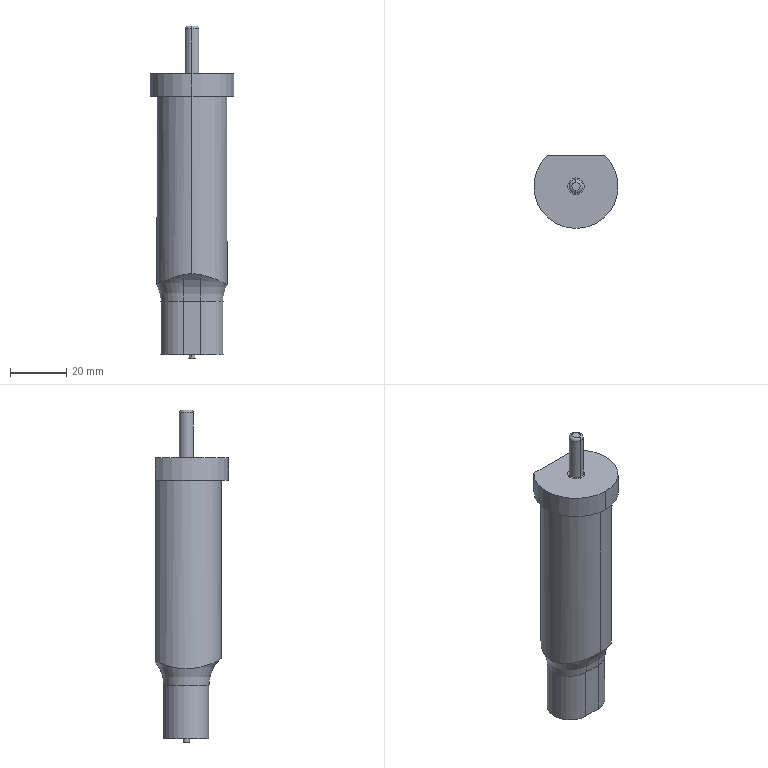Part | STEP file | 1_id3566_x_t | 1 solid | 27 faces | box 30 x 26 x 118.2 mm | volume 45235 mm3 | cylinder 14 | plane 9 | torus 4 | commonest cylinder face diameters 2.26 x2 5 x2 6 x2 16.07 x2 25 x2 26 x2
STEP:
#1=CARTESIAN_POINT('',(3206.065,143.382,20.96));
#2=VERTEX_POINT('',#1);
#3=CARTESIAN_POINT('',(3208.937,166.5,20.193));
#4=VERTEX_POINT('',#3);
#5=CARTESIAN_POINT('',(3206.065,143.382,20.96));
#6=CARTESIAN_POINT('',(3208.507,143.999,20.378));
#7=CARTESIAN_POINT('',(3210.679,145.334,19.684));
#8=CARTESIAN_POINT('',(3213.962,149.007,18.317));
#9=CARTESIAN_POINT('',(3215.071,151.383,17.64));
#10=CARTESIAN_POINT('',(3215.722,156.404,17.229));
#11=CARTESIAN_POINT('',(3215.235,159.073,17.588));
#12=CARTESIAN_POINT('',(3212.932,163.488,18.779));
#13=CARTESIAN_POINT('',(3211.138,165.312,19.533));
#14=CARTESIAN_POINT('',(3208.937,166.5,20.193));
#15=B_SPLINE_CURVE_WITH_KNOTS('',3,(#5,#6,#7,#8,#9,#10,#11,#12,#13,#14),.UNSPECIFIED.,.F.,.F.,(4,2,2,2,4),(0.,0.25,0.5,0.75,1.),.UNSPECIFIED.);
#16=EDGE_CURVE('',#2,#4,#15,.T.);
#17=ORIENTED_EDGE('',*,*,#16,.T.);
#18=CARTESIAN_POINT('',(3208.937,166.5,84.5));
#19=VERTEX_POINT('',#18);
#20=CARTESIAN_POINT('',(3208.937,166.5,38.5));
#21=DIRECTION('',(0.,0.,1.));
#22=VECTOR('',#21,1.);
#23=LINE('',#20,#22);
#24=EDGE_CURVE('',#4,#19,#23,.T.);
#25=ORIENTED_EDGE('',*,*,#24,.T.);
#26=CARTESIAN_POINT('',(3203.,143.,84.5));
#27=VERTEX_POINT('',#26);
#28=CARTESIAN_POINT('',(3203.,155.5,84.5));
#29=DIRECTION('',(0.,0.,1.));
#30=DIRECTION('',(0.,-1.,0.));
#31=AXIS2_PLACEMENT_3D('',#28,#29,#30);
#32=CIRCLE('',#31,12.5);
#33=EDGE_CURVE('',#27,#19,#32,.T.);
#34=ORIENTED_EDGE('',*,*,#33,.F.);
#35=CARTESIAN_POINT('',(3203.,143.,21.306));
#36=VERTEX_POINT('',#35);
#37=CARTESIAN_POINT('',(3203.,143.,38.5));
#38=DIRECTION('',(0.,0.,1.));
#39=VECTOR('',#38,1.);
#40=LINE('',#37,#39);
#41=EDGE_CURVE('',#36,#27,#40,.T.);
#42=ORIENTED_EDGE('',*,*,#41,.F.);
#43=CARTESIAN_POINT('',(3203.,143.,21.306));
#44=CARTESIAN_POINT('',(3204.051,143.,21.306));
#45=CARTESIAN_POINT('',(3205.073,143.131,21.197));
#46=CARTESIAN_POINT('',(3206.065,143.382,20.96));
#47=B_SPLINE_CURVE_WITH_KNOTS('',3,(#43,#44,#45,#46),.UNSPECIFIED.,.F.,.F.,(4,4),(0.,1.),.UNSPECIFIED.);
#48=EDGE_CURVE('',#36,#2,#47,.T.);
#49=ORIENTED_EDGE('',*,*,#48,.T.);
#50=EDGE_LOOP('',(#17,#25,#34,#42,#49));
#51=FACE_OUTER_BOUND('',#50,.T.);
#52=CARTESIAN_POINT('',(3203.,155.5,38.5));
#53=DIRECTION('',(0.,0.,-1.));
#54=DIRECTION('',(0.,1.,0.));
#55=AXIS2_PLACEMENT_3D('',#52,#53,#54);
#56=CYLINDRICAL_SURFACE('',#55,12.5);
#57=ADVANCED_FACE('',(#51),#56,.T.);
#58=CARTESIAN_POINT('',(3203.,140.5,84.5));
#59=VERTEX_POINT('',#58);
#60=CARTESIAN_POINT('',(3213.198,166.5,84.5));
#61=VERTEX_POINT('',#60);
#62=CARTESIAN_POINT('',(3203.,155.5,84.5));
#63=DIRECTION('',(0.,0.,1.));
#64=DIRECTION('',(0.,-1.,0.));
#65=AXIS2_PLACEMENT_3D('',#62,#63,#64);
#66=CIRCLE('',#65,15.);
#67=EDGE_CURVE('',#59,#61,#66,.T.);
#68=ORIENTED_EDGE('',*,*,#67,.T.);
#69=CARTESIAN_POINT('',(3213.198,166.5,92.5));
#70=VERTEX_POINT('',#69);
#71=CARTESIAN_POINT('',(3213.198,166.5,88.5));
#72=DIRECTION('',(0.,0.,1.));
#73=VECTOR('',#72,1.);
#74=LINE('',#71,#73);
#75=EDGE_CURVE('',#61,#70,#74,.T.);
#76=ORIENTED_EDGE('',*,*,#75,.T.);
#77=CARTESIAN_POINT('',(3203.,140.5,92.5));
#78=VERTEX_POINT('',#77);
#79=CARTESIAN_POINT('',(3203.,155.5,92.5));
#80=DIRECTION('',(0.,0.,1.));
#81=DIRECTION('',(0.,-1.,0.));
#82=AXIS2_PLACEMENT_3D('',#79,#80,#81);
#83=CIRCLE('',#82,15.);
#84=EDGE_CURVE('',#78,#70,#83,.T.);
#85=ORIENTED_EDGE('',*,*,#84,.F.);
#86=CARTESIAN_POINT('',(3203.,140.5,88.5));
#87=DIRECTION('',(0.,0.,1.));
#88=VECTOR('',#87,1.);
#89=LINE('',#86,#88);
#90=EDGE_CURVE('',#59,#78,#89,.T.);
#91=ORIENTED_EDGE('',*,*,#90,.F.);
#92=EDGE_LOOP('',(#68,#76,#85,#91));
#93=FACE_OUTER_BOUND('',#92,.T.);
#94=CARTESIAN_POINT('',(3203.,155.5,88.5));
#95=DIRECTION('',(0.,0.,-1.));
#96=DIRECTION('',(0.,1.,0.));
#97=AXIS2_PLACEMENT_3D('',#94,#95,#96);
#98=CYLINDRICAL_SURFACE('',#97,15.);
#99=ADVANCED_FACE('',(#93),#98,.T.);
#100=CARTESIAN_POINT('',(3192.802,166.5,92.5));
#101=VERTEX_POINT('',#100);
#102=CARTESIAN_POINT('',(3203.,155.5,92.5));
#103=DIRECTION('',(0.,0.,1.));
#104=DIRECTION('',(0.,-1.,0.));
#105=AXIS2_PLACEMENT_3D('',#102,#103,#104);
#106=CIRCLE('',#105,15.);
#107=EDGE_CURVE('',#101,#78,#106,.T.);
#108=ORIENTED_EDGE('',*,*,#107,.F.);
#109=CARTESIAN_POINT('',(3192.802,166.5,84.5));
#110=VERTEX_POINT('',#109);
#111=CARTESIAN_POINT('',(3192.802,166.5,88.5));
#112=DIRECTION('',(0.,0.,1.));
#113=VECTOR('',#112,1.);
#114=LINE('',#111,#113);
#115=EDGE_CURVE('',#110,#101,#114,.T.);
#116=ORIENTED_EDGE('',*,*,#115,.F.);
#117=CARTESIAN_POINT('',(3203.,155.5,84.5));
#118=DIRECTION('',(0.,0.,1.));
#119=DIRECTION('',(0.,-1.,0.));
#120=AXIS2_PLACEMENT_3D('',#117,#118,#119);
#121=CIRCLE('',#120,15.);
#122=EDGE_CURVE('',#110,#59,#121,.T.);
#123=ORIENTED_EDGE('',*,*,#122,.T.);
#124=ORIENTED_EDGE('',*,*,#90,.T.);
#125=EDGE_LOOP('',(#108,#116,#123,#124));
#126=FACE_OUTER_BOUND('',#125,.T.);
#127=CARTESIAN_POINT('',(3203.,155.5,88.5));
#128=DIRECTION('',(0.,0.,-1.));
#129=DIRECTION('',(0.,1.,0.));
#130=AXIS2_PLACEMENT_3D('',#127,#128,#129);
#131=CYLINDRICAL_SURFACE('',#130,15.);
#132=ADVANCED_FACE('',(#126),#131,.T.);
#133=ORIENTED_EDGE('',*,*,#122,.F.);
#134=CARTESIAN_POINT('',(3197.063,166.5,84.5));
#135=VERTEX_POINT('',#134);
#136=CARTESIAN_POINT('',(3203.,166.5,84.5));
#137=DIRECTION('',(-1.,0.,0.));
#138=VECTOR('',#137,1.);
#139=LINE('',#136,#138);
#140=EDGE_CURVE('',#135,#110,#139,.T.);
#141=ORIENTED_EDGE('',*,*,#140,.F.);
#142=CARTESIAN_POINT('',(3203.,155.5,84.5));
#143=DIRECTION('',(0.,0.,1.));
#144=DIRECTION('',(0.,-1.,0.));
#145=AXIS2_PLACEMENT_3D('',#142,#143,#144);
#146=CIRCLE('',#145,12.5);
#147=EDGE_CURVE('',#135,#27,#146,.T.);
#148=ORIENTED_EDGE('',*,*,#147,.T.);
#149=ORIENTED_EDGE('',*,*,#33,.T.);
#150=CARTESIAN_POINT('',(3203.,166.5,84.5));
#151=DIRECTION('',(-1.,0.,0.));
#152=VECTOR('',#151,1.);
#153=LINE('',#150,#152);
#154=EDGE_CURVE('',#61,#19,#153,.T.);
#155=ORIENTED_EDGE('',*,*,#154,.F.);
#156=ORIENTED_EDGE('',*,*,#67,.F.);
#157=EDGE_LOOP('',(#133,#141,#148,#149,#155,#156));
#158=FACE_OUTER_BOUND('',#157,.T.);
#159=CARTESIAN_POINT('',(3203.,141.75,84.5));
#160=DIRECTION('',(0.,0.,-1.));
#161=DIRECTION('',(0.,-1.,0.));
#162=AXIS2_PLACEMENT_3D('',#159,#160,#161);
#163=PLANE('',#162);
#164=ADVANCED_FACE('',(#158),#163,.T.);
#165=CARTESIAN_POINT('',(3206.065,166.5,19.764));
#166=VERTEX_POINT('',#165);
#167=CARTESIAN_POINT('',(3206.065,166.5,19.764));
#168=CARTESIAN_POINT('',(3207.044,166.5,19.764));
#169=CARTESIAN_POINT('',(3207.998,166.5,19.929));
#170=CARTESIAN_POINT('',(3208.937,166.5,20.193));
#171=B_SPLINE_CURVE_WITH_KNOTS('',3,(#167,#168,#169,#170),.UNSPECIFIED.,.F.,.F.,(4,4),(0.,1.),.UNSPECIFIED.);
#172=EDGE_CURVE('',#166,#4,#171,.T.);
#173=ORIENTED_EDGE('',*,*,#172,.T.);
#174=ORIENTED_EDGE('',*,*,#16,.F.);
#175=CARTESIAN_POINT('',(3206.065,147.465,11.5));
#176=VERTEX_POINT('',#175);
#177=CARTESIAN_POINT('',(3206.065,134.465,11.5));
#178=DIRECTION('',(-1.,0.,0.));
#179=DIRECTION('',(0.,-1.,0.));
#180=AXIS2_PLACEMENT_3D('',#177,#178,#179);
#181=CIRCLE('',#180,13.);
#182=EDGE_CURVE('',#2,#176,#181,.T.);
#183=ORIENTED_EDGE('',*,*,#182,.T.);
#184=CARTESIAN_POINT('',(3206.065,163.535,11.5));
#185=VERTEX_POINT('',#184);
#186=CARTESIAN_POINT('',(3206.065,155.5,11.5));
#187=DIRECTION('',(0.,0.,-1.));
#188=DIRECTION('',(0.,1.,0.));
#189=AXIS2_PLACEMENT_3D('',#186,#187,#188);
#190=CIRCLE('',#189,8.035);
#191=EDGE_CURVE('',#185,#176,#190,.T.);
#192=ORIENTED_EDGE('',*,*,#191,.F.);
#193=CARTESIAN_POINT('',(3206.065,176.535,11.5));
#194=DIRECTION('',(1.,0.,0.));
#195=DIRECTION('',(0.,1.,0.));
#196=AXIS2_PLACEMENT_3D('',#193,#194,#195);
#197=CIRCLE('',#196,13.);
#198=EDGE_CURVE('',#166,#185,#197,.T.);
#199=ORIENTED_EDGE('',*,*,#198,.F.);
#200=EDGE_LOOP('',(#173,#174,#183,#192,#199));
#201=FACE_OUTER_BOUND('',#200,.T.);
#202=CARTESIAN_POINT('',(3206.065,155.5,11.5));
#203=DIRECTION('',(0.,0.,-1.));
#204=DIRECTION('',(0.,1.,0.));
#205=AXIS2_PLACEMENT_3D('',#202,#203,#204);
#206=TOROIDAL_SURFACE('',#205,21.035,13.);
#207=ADVANCED_FACE('',(#201),#206,.F.);
#208=CARTESIAN_POINT('',(3199.935,166.5,19.764));
#209=VERTEX_POINT('',#208);
#210=CARTESIAN_POINT('',(3178.,166.5,19.764));
#211=DIRECTION('',(-1.,0.,0.));
#212=VECTOR('',#211,1.);
#213=LINE('',#210,#212);
#214=EDGE_CURVE('',#166,#209,#213,.T.);
#215=ORIENTED_EDGE('',*,*,#214,.F.);
#216=ORIENTED_EDGE('',*,*,#198,.T.);
#217=CARTESIAN_POINT('',(3199.935,163.535,11.5));
#218=VERTEX_POINT('',#217);
#219=CARTESIAN_POINT('',(3178.,163.535,11.5));
#220=DIRECTION('',(1.,0.,0.));
#221=VECTOR('',#220,1.);
#222=LINE('',#219,#221);
#223=EDGE_CURVE('',#218,#185,#222,.T.);
#224=ORIENTED_EDGE('',*,*,#223,.F.);
#225=CARTESIAN_POINT('',(3199.935,176.535,11.5));
#226=DIRECTION('',(-1.,0.,0.));
#227=DIRECTION('',(0.,1.,0.));
#228=AXIS2_PLACEMENT_3D('',#225,#226,#227);
#229=CIRCLE('',#228,13.);
#230=EDGE_CURVE('',#218,#209,#229,.T.);
#231=ORIENTED_EDGE('',*,*,#230,.T.);
#232=EDGE_LOOP('',(#215,#216,#224,#231));
#233=FACE_OUTER_BOUND('',#232,.T.);
#234=CARTESIAN_POINT('',(3178.,176.535,11.5));
#235=DIRECTION('',(-1.,0.,0.));
#236=DIRECTION('',(0.,1.,0.));
#237=AXIS2_PLACEMENT_3D('',#234,#235,#236);
#238=CYLINDRICAL_SURFACE('',#237,13.);
#239=ADVANCED_FACE('',(#233),#238,.F.);
#240=CARTESIAN_POINT('',(3197.063,166.5,20.193));
#241=VERTEX_POINT('',#240);
#242=CARTESIAN_POINT('',(3197.063,166.5,20.193));
#243=CARTESIAN_POINT('',(3198.002,166.5,19.929));
#244=CARTESIAN_POINT('',(3198.956,166.5,19.764));
#245=CARTESIAN_POINT('',(3199.935,166.5,19.764));
#246=B_SPLINE_CURVE_WITH_KNOTS('',3,(#242,#243,#244,#245),.UNSPECIFIED.,.F.,.F.,(4,4),(0.,1.),.UNSPECIFIED.);
#247=EDGE_CURVE('',#241,#209,#246,.T.);
#248=ORIENTED_EDGE('',*,*,#247,.T.);
#249=ORIENTED_EDGE('',*,*,#230,.F.);
#250=CARTESIAN_POINT('',(3199.935,147.465,11.5));
#251=VERTEX_POINT('',#250);
#252=CARTESIAN_POINT('',(3199.935,155.5,11.5));
#253=DIRECTION('',(0.,0.,1.));
#254=DIRECTION('',(0.,1.,0.));
#255=AXIS2_PLACEMENT_3D('',#252,#253,#254);
#256=CIRCLE('',#255,8.035);
#257=EDGE_CURVE('',#218,#251,#256,.T.);
#258=ORIENTED_EDGE('',*,*,#257,.T.);
#259=CARTESIAN_POINT('',(3199.935,143.382,20.96));
#260=VERTEX_POINT('',#259);
#261=CARTESIAN_POINT('',(3199.935,134.465,11.5));
#262=DIRECTION('',(1.,0.,0.));
#263=DIRECTION('',(0.,-1.,0.));
#264=AXIS2_PLACEMENT_3D('',#261,#262,#263);
#265=CIRCLE('',#264,13.);
#266=EDGE_CURVE('',#251,#260,#265,.T.);
#267=ORIENTED_EDGE('',*,*,#266,.T.);
#268=CARTESIAN_POINT('',(3197.063,166.5,20.193));
#269=CARTESIAN_POINT('',(3194.864,165.313,19.534));
#270=CARTESIAN_POINT('',(3193.084,163.505,18.786));
#271=CARTESIAN_POINT('',(3190.778,159.111,17.596));
#272=CARTESIAN_POINT('',(3190.28,156.461,17.23));
#273=CARTESIAN_POINT('',(3190.916,151.414,17.632));
#274=CARTESIAN_POINT('',(3192.028,149.025,18.311));
#275=CARTESIAN_POINT('',(3195.303,145.348,19.678));
#276=CARTESIAN_POINT('',(3197.491,144.,20.378));
#277=CARTESIAN_POINT('',(3199.935,143.382,20.96));
#278=B_SPLINE_CURVE_WITH_KNOTS('',3,(#268,#269,#270,#271,#272,#273,#274,#275,#276,#277),.UNSPECIFIED.,.F.,.F.,(4,2,2,2,4),(0.,0.25,0.5,0.75,1.),.UNSPECIFIED.);
#279=EDGE_CURVE('',#241,#260,#278,.T.);
#280=ORIENTED_EDGE('',*,*,#279,.F.);
#281=EDGE_LOOP('',(#248,#249,#258,#267,#280));
#282=FACE_OUTER_BOUND('',#281,.T.);
#283=CARTESIAN_POINT('',(3199.935,155.5,11.5));
#284=DIRECTION('',(0.,0.,1.));
#285=DIRECTION('',(0.,-1.,0.));
#286=AXIS2_PLACEMENT_3D('',#283,#284,#285);
#287=TOROIDAL_SURFACE('',#286,21.035,13.);
#288=ADVANCED_FACE('',(#282),#287,.F.);
#289=ORIENTED_EDGE('',*,*,#147,.F.);
#290=CARTESIAN_POINT('',(3197.063,166.5,38.5));
#291=DIRECTION('',(0.,0.,-1.));
#292=VECTOR('',#291,1.);
#293=LINE('',#290,#292);
#294=EDGE_CURVE('',#135,#241,#293,.T.);
#295=ORIENTED_EDGE('',*,*,#294,.T.);
#296=ORIENTED_EDGE('',*,*,#279,.T.);
#297=CARTESIAN_POINT('',(3199.935,143.382,20.96));
#298=CARTESIAN_POINT('',(3200.928,143.131,21.197));
#299=CARTESIAN_POINT('',(3201.95,143.,21.306));
#300=CARTESIAN_POINT('',(3203.,143.,21.306));
#301=B_SPLINE_CURVE_WITH_KNOTS('',3,(#297,#298,#299,#300),.UNSPECIFIED.,.F.,.F.,(4,4),(0.,1.),.UNSPECIFIED.);
#302=EDGE_CURVE('',#260,#36,#301,.T.);
#303=ORIENTED_EDGE('',*,*,#302,.T.);
#304=ORIENTED_EDGE('',*,*,#41,.T.);
#305=EDGE_LOOP('',(#289,#295,#296,#303,#304));
#306=FACE_OUTER_BOUND('',#305,.T.);
#307=CARTESIAN_POINT('',(3203.,155.5,38.5));
#308=DIRECTION('',(0.,0.,-1.));
#309=DIRECTION('',(0.,1.,0.));
#310=AXIS2_PLACEMENT_3D('',#307,#308,#309);
#311=CYLINDRICAL_SURFACE('',#310,12.5);
#312=ADVANCED_FACE('',(#306),#311,.T.);
#313=CARTESIAN_POINT('',(3203.,152.5,92.5));
#314=VERTEX_POINT('',#313);
#315=CARTESIAN_POINT('',(3203.,158.5,92.5));
#316=VERTEX_POINT('',#315);
#317=CARTESIAN_POINT('',(3203.,155.5,92.5));
#318=DIRECTION('',(0.,0.,-1.));
#319=DIRECTION('',(0.,1.,0.));
#320=AXIS2_PLACEMENT_3D('',#317,#318,#319);
#321=CIRCLE('',#320,3.);
#322=EDGE_CURVE('',#314,#316,#321,.T.);
#323=ORIENTED_EDGE('',*,*,#322,.T.);
#324=CARTESIAN_POINT('',(3203.,155.5,92.5));
#325=DIRECTION('',(0.,0.,-1.));
#326=DIRECTION('',(0.,1.,0.));
#327=AXIS2_PLACEMENT_3D('',#324,#325,#326);
#328=CIRCLE('',#327,3.);
#329=EDGE_CURVE('',#316,#314,#328,.T.);
#330=ORIENTED_EDGE('',*,*,#329,.T.);
#331=EDGE_LOOP('',(#323,#330));
#332=FACE_BOUND('',#331,.T.);
#333=ORIENTED_EDGE('',*,*,#84,.T.);
#334=CARTESIAN_POINT('',(3203.,166.5,92.5));
#335=DIRECTION('',(-1.,0.,0.));
#336=VECTOR('',#335,1.);
#337=LINE('',#334,#336);
#338=EDGE_CURVE('',#70,#101,#337,.T.);
#339=ORIENTED_EDGE('',*,*,#338,.T.);
#340=ORIENTED_EDGE('',*,*,#107,.T.);
#341=EDGE_LOOP('',(#333,#339,#340));
#342=FACE_BOUND('',#341,.T.);
#343=CARTESIAN_POINT('',(3203.,148.,92.5));
#344=DIRECTION('',(0.,0.,1.));
#345=DIRECTION('',(0.,1.,0.));
#346=AXIS2_PLACEMENT_3D('',#343,#344,#345);
#347=PLANE('',#346);
#348=ADVANCED_FACE('',(#332,#342),#347,.T.);
#349=CARTESIAN_POINT('',(3203.,156.63,-7.5));
#350=VERTEX_POINT('',#349);
#351=CARTESIAN_POINT('',(3203.,156.63,-8.7));
#352=VERTEX_POINT('',#351);
#353=CARTESIAN_POINT('',(3203.,156.63,-7.5));
#354=DIRECTION('',(0.,0.,-1.));
#355=VECTOR('',#354,1.);
#356=LINE('',#353,#355);
#357=EDGE_CURVE('',#350,#352,#356,.T.);
#358=ORIENTED_EDGE('',*,*,#357,.F.);
#359=CARTESIAN_POINT('',(3203.,154.37,-7.5));
#360=VERTEX_POINT('',#359);
#361=CARTESIAN_POINT('',(3203.,155.5,-7.5));
#362=DIRECTION('',(0.,0.,1.));
#363=DIRECTION('',(0.,1.,0.));
#364=AXIS2_PLACEMENT_3D('',#361,#362,#363);
#365=CIRCLE('',#364,1.13);
#366=EDGE_CURVE('',#360,#350,#365,.T.);
#367=ORIENTED_EDGE('',*,*,#366,.F.);
#368=CARTESIAN_POINT('',(3203.,154.37,-8.7));
#369=VERTEX_POINT('',#368);
#370=CARTESIAN_POINT('',(3203.,154.37,-7.5));
#371=DIRECTION('',(0.,0.,1.));
#372=VECTOR('',#371,1.);
#373=LINE('',#370,#372);
#374=EDGE_CURVE('',#369,#360,#373,.T.);
#375=ORIENTED_EDGE('',*,*,#374,.F.);
#376=CARTESIAN_POINT('',(3203.,155.5,-8.7));
#377=DIRECTION('',(0.,0.,1.));
#378=DIRECTION('',(0.,1.,0.));
#379=AXIS2_PLACEMENT_3D('',#376,#377,#378);
#380=CIRCLE('',#379,1.13);
#381=EDGE_CURVE('',#369,#352,#380,.T.);
#382=ORIENTED_EDGE('',*,*,#381,.T.);
#383=EDGE_LOOP('',(#358,#367,#375,#382));
#384=FACE_OUTER_BOUND('',#383,.T.);
#385=CARTESIAN_POINT('',(3203.,155.5,-7.5));
#386=DIRECTION('',(0.,0.,1.));
#387=DIRECTION('',(0.,-1.,0.));
#388=AXIS2_PLACEMENT_3D('',#385,#386,#387);
#389=CYLINDRICAL_SURFACE('',#388,1.13);
#390=ADVANCED_FACE('',(#384),#389,.T.);
#391=CARTESIAN_POINT('',(3203.,158.,108.5));
#392=VERTEX_POINT('',#391);
#393=CARTESIAN_POINT('',(3203.,158.,92.6));
#394=VERTEX_POINT('',#393);
#395=CARTESIAN_POINT('',(3203.,158.,100.55));
#396=DIRECTION('',(0.,0.,-1.));
#397=VECTOR('',#396,1.);
#398=LINE('',#395,#397);
#399=EDGE_CURVE('',#392,#394,#398,.T.);
#400=ORIENTED_EDGE('',*,*,#399,.F.);
#401=CARTESIAN_POINT('',(3203.,153.,108.5));
#402=VERTEX_POINT('',#401);
#403=CARTESIAN_POINT('',(3203.,155.5,108.5));
#404=DIRECTION('',(0.,0.,-1.));
#405=DIRECTION('',(0.,1.,0.));
#406=AXIS2_PLACEMENT_3D('',#403,#404,#405);
#407=CIRCLE('',#406,2.5);
#408=EDGE_CURVE('',#392,#402,#407,.T.);
#409=ORIENTED_EDGE('',*,*,#408,.T.);
#410=CARTESIAN_POINT('',(3203.,153.,92.6));
#411=VERTEX_POINT('',#410);
#412=CARTESIAN_POINT('',(3203.,153.,100.55));
#413=DIRECTION('',(0.,0.,1.));
#414=VECTOR('',#413,1.);
#415=LINE('',#412,#414);
#416=EDGE_CURVE('',#411,#402,#415,.T.);
#417=ORIENTED_EDGE('',*,*,#416,.F.);
#418=CARTESIAN_POINT('',(3203.,155.5,92.6));
#419=DIRECTION('',(0.,0.,-1.));
#420=DIRECTION('',(0.,1.,0.));
#421=AXIS2_PLACEMENT_3D('',#418,#419,#420);
#422=CIRCLE('',#421,2.5);
#423=EDGE_CURVE('',#394,#411,#422,.T.);
#424=ORIENTED_EDGE('',*,*,#423,.F.);
#425=EDGE_LOOP('',(#400,#409,#417,#424));
#426=FACE_OUTER_BOUND('',#425,.T.);
#427=CARTESIAN_POINT('',(3203.,155.5,100.55));
#428=DIRECTION('',(0.,0.,1.));
#429=DIRECTION('',(0.,-1.,0.));
#430=AXIS2_PLACEMENT_3D('',#427,#428,#429);
#431=CYLINDRICAL_SURFACE('',#430,2.5);
#432=ADVANCED_FACE('',(#426),#431,.T.);
#433=CARTESIAN_POINT('',(3203.,154.,109.5));
#434=VERTEX_POINT('',#433);
#435=CARTESIAN_POINT('',(3203.,154.,108.5));
#436=DIRECTION('',(1.,0.,0.));
#437=DIRECTION('',(0.,-1.,0.));
#438=AXIS2_PLACEMENT_3D('',#435,#436,#437);
#439=CIRCLE('',#438,1.);
#440=EDGE_CURVE('',#434,#402,#439,.T.);
#441=ORIENTED_EDGE('',*,*,#440,.F.);
#442=CARTESIAN_POINT('',(3203.,157.,109.5));
#443=VERTEX_POINT('',#442);
#444=CARTESIAN_POINT('',(3203.,155.5,109.5));
#445=DIRECTION('',(0.,0.,-1.));
#446=DIRECTION('',(0.,1.,0.));
#447=AXIS2_PLACEMENT_3D('',#444,#445,#446);
#448=CIRCLE('',#447,1.5);
#449=EDGE_CURVE('',#434,#443,#448,.T.);
#450=ORIENTED_EDGE('',*,*,#449,.T.);
#451=CARTESIAN_POINT('',(3203.,157.,108.5));
#452=DIRECTION('',(1.,0.,0.));
#453=DIRECTION('',(0.,1.,0.));
#454=AXIS2_PLACEMENT_3D('',#451,#452,#453);
#455=CIRCLE('',#454,1.);
#456=EDGE_CURVE('',#392,#443,#455,.T.);
#457=ORIENTED_EDGE('',*,*,#456,.F.);
#458=CARTESIAN_POINT('',(3203.,155.5,108.5));
#459=DIRECTION('',(0.,0.,-1.));
#460=DIRECTION('',(0.,1.,0.));
#461=AXIS2_PLACEMENT_3D('',#458,#459,#460);
#462=CIRCLE('',#461,2.5);
#463=EDGE_CURVE('',#402,#392,#462,.T.);
#464=ORIENTED_EDGE('',*,*,#463,.F.);
#465=EDGE_LOOP('',(#441,#450,#457,#464));
#466=FACE_OUTER_BOUND('',#465,.T.);
#467=CARTESIAN_POINT('',(3203.,155.5,108.5));
#468=DIRECTION('',(0.,0.,-1.));
#469=DIRECTION('',(0.,1.,0.));
#470=AXIS2_PLACEMENT_3D('',#467,#468,#469);
#471=TOROIDAL_SURFACE('',#470,1.5,1.);
#472=ADVANCED_FACE('',(#466),#471,.T.);
#473=CARTESIAN_POINT('',(3203.,158.5,92.6));
#474=VERTEX_POINT('',#473);
#475=CARTESIAN_POINT('',(3203.,158.5,92.55));
#476=DIRECTION('',(0.,0.,-1.));
#477=VECTOR('',#476,1.);
#478=LINE('',#475,#477);
#479=EDGE_CURVE('',#474,#316,#478,.T.);
#480=ORIENTED_EDGE('',*,*,#479,.F.);
#481=CARTESIAN_POINT('',(3203.,152.5,92.6));
#482=VERTEX_POINT('',#481);
#483=CARTESIAN_POINT('',(3203.,155.5,92.6));
#484=DIRECTION('',(0.,0.,-1.));
#485=DIRECTION('',(0.,1.,0.));
#486=AXIS2_PLACEMENT_3D('',#483,#484,#485);
#487=CIRCLE('',#486,3.);
#488=EDGE_CURVE('',#474,#482,#487,.T.);
#489=ORIENTED_EDGE('',*,*,#488,.T.);
#490=CARTESIAN_POINT('',(3203.,152.5,92.55));
#491=DIRECTION('',(0.,0.,1.));
#492=VECTOR('',#491,1.);
#493=LINE('',#490,#492);
#494=EDGE_CURVE('',#314,#482,#493,.T.);
#495=ORIENTED_EDGE('',*,*,#494,.F.);
#496=ORIENTED_EDGE('',*,*,#329,.F.);
#497=EDGE_LOOP('',(#480,#489,#495,#496));
#498=FACE_OUTER_BOUND('',#497,.T.);
#499=CARTESIAN_POINT('',(3203.,155.5,87.05));
#500=DIRECTION('',(0.,0.,1.));
#501=DIRECTION('',(0.,-1.,0.));
#502=AXIS2_PLACEMENT_3D('',#499,#500,#501);
#503=CYLINDRICAL_SURFACE('',#502,3.);
#504=ADVANCED_FACE('',(#498),#503,.T.);
#505=ORIENTED_EDGE('',*,*,#479,.T.);
#506=ORIENTED_EDGE('',*,*,#322,.F.);
#507=ORIENTED_EDGE('',*,*,#494,.T.);
#508=CARTESIAN_POINT('',(3203.,155.5,92.6));
#509=DIRECTION('',(0.,0.,-1.));
#510=DIRECTION('',(0.,1.,0.));
#511=AXIS2_PLACEMENT_3D('',#508,#509,#510);
#512=CIRCLE('',#511,3.);
#513=EDGE_CURVE('',#482,#474,#512,.T.);
#514=ORIENTED_EDGE('',*,*,#513,.T.);
#515=EDGE_LOOP('',(#505,#506,#507,#514));
#516=FACE_OUTER_BOUND('',#515,.T.);
#517=CARTESIAN_POINT('',(3203.,155.5,87.05));
#518=DIRECTION('',(0.,0.,1.));
#519=DIRECTION('',(0.,-1.,0.));
#520=AXIS2_PLACEMENT_3D('',#517,#518,#519);
#521=CYLINDRICAL_SURFACE('',#520,3.);
#522=ADVANCED_FACE('',(#516),#521,.T.);
#523=CARTESIAN_POINT('',(3203.,155.5,109.5));
#524=DIRECTION('',(0.,0.,-1.));
#525=DIRECTION('',(0.,1.,0.));
#526=AXIS2_PLACEMENT_3D('',#523,#524,#525);
#527=CIRCLE('',#526,1.5);
#528=EDGE_CURVE('',#443,#434,#527,.T.);
#529=ORIENTED_EDGE('',*,*,#528,.F.);
#530=ORIENTED_EDGE('',*,*,#449,.F.);
#531=EDGE_LOOP('',(#529,#530));
#532=FACE_OUTER_BOUND('',#531,.T.);
#533=CARTESIAN_POINT('',(3203.,156.25,109.5));
#534=DIRECTION('',(0.,0.,1.));
#535=DIRECTION('',(0.,1.,0.));
#536=AXIS2_PLACEMENT_3D('',#533,#534,#535);
#537=PLANE('',#536);
#538=ADVANCED_FACE('',(#532),#537,.T.);
#539=ORIENTED_EDGE('',*,*,#440,.T.);
#540=ORIENTED_EDGE('',*,*,#408,.F.);
#541=ORIENTED_EDGE('',*,*,#456,.T.);
#542=ORIENTED_EDGE('',*,*,#528,.T.);
#543=EDGE_LOOP('',(#539,#540,#541,#542));
#544=FACE_OUTER_BOUND('',#543,.T.);
#545=CARTESIAN_POINT('',(3203.,155.5,108.5));
#546=DIRECTION('',(0.,0.,-1.));
#547=DIRECTION('',(0.,1.,0.));
#548=AXIS2_PLACEMENT_3D('',#545,#546,#547);
#549=TOROIDAL_SURFACE('',#548,1.5,1.);
#550=ADVANCED_FACE('',(#544),#549,.T.);
#551=ORIENTED_EDGE('',*,*,#399,.T.);
#552=CARTESIAN_POINT('',(3203.,155.5,92.6));
#553=DIRECTION('',(0.,0.,-1.));
#554=DIRECTION('',(0.,1.,0.));
#555=AXIS2_PLACEMENT_3D('',#552,#553,#554);
#556=CIRCLE('',#555,2.5);
#557=EDGE_CURVE('',#411,#394,#556,.T.);
#558=ORIENTED_EDGE('',*,*,#557,.F.);
#559=ORIENTED_EDGE('',*,*,#416,.T.);
#560=ORIENTED_EDGE('',*,*,#463,.T.);
#561=EDGE_LOOP('',(#551,#558,#559,#560));
#562=FACE_OUTER_BOUND('',#561,.T.);
#563=CARTESIAN_POINT('',(3203.,155.5,100.55));
#564=DIRECTION('',(0.,0.,1.));
#565=DIRECTION('',(0.,-1.,0.));
#566=AXIS2_PLACEMENT_3D('',#563,#564,#565);
#567=CYLINDRICAL_SURFACE('',#566,2.5);
#568=ADVANCED_FACE('',(#562),#567,.T.);
#569=ORIENTED_EDGE('',*,*,#488,.F.);
#570=ORIENTED_EDGE('',*,*,#513,.F.);
#571=EDGE_LOOP('',(#569,#570));
#572=FACE_BOUND('',#571,.T.);
#573=ORIENTED_EDGE('',*,*,#423,.T.);
#574=ORIENTED_EDGE('',*,*,#557,.T.);
#575=EDGE_LOOP('',(#573,#574));
#576=FACE_BOUND('',#575,.T.);
#577=CARTESIAN_POINT('',(3203.,158.25,92.6));
#578=DIRECTION('',(0.,0.,1.));
#579=DIRECTION('',(0.,1.,0.));
#580=AXIS2_PLACEMENT_3D('',#577,#578,#579);
#581=PLANE('',#580);
#582=ADVANCED_FACE('',(#572,#576),#581,.T.);
#583=ORIENTED_EDGE('',*,*,#357,.T.);
#584=CARTESIAN_POINT('',(3203.,155.5,-8.7));
#585=DIRECTION('',(0.,0.,1.));
#586=DIRECTION('',(0.,1.,0.));
#587=AXIS2_PLACEMENT_3D('',#584,#585,#586);
#588=CIRCLE('',#587,1.13);
#589=EDGE_CURVE('',#352,#369,#588,.T.);
#590=ORIENTED_EDGE('',*,*,#589,.T.);
#591=ORIENTED_EDGE('',*,*,#374,.T.);
#592=CARTESIAN_POINT('',(3203.,155.5,-7.5));
#593=DIRECTION('',(0.,0.,1.));
#594=DIRECTION('',(0.,1.,0.));
#595=AXIS2_PLACEMENT_3D('',#592,#593,#594);
#596=CIRCLE('',#595,1.13);
#597=EDGE_CURVE('',#350,#360,#596,.T.);
#598=ORIENTED_EDGE('',*,*,#597,.F.);
#599=EDGE_LOOP('',(#583,#590,#591,#598));
#600=FACE_OUTER_BOUND('',#599,.T.);
#601=CARTESIAN_POINT('',(3203.,155.5,-7.5));
#602=DIRECTION('',(0.,0.,1.));
#603=DIRECTION('',(0.,-1.,0.));
#604=AXIS2_PLACEMENT_3D('',#601,#602,#603);
#605=CYLINDRICAL_SURFACE('',#604,1.13);
#606=ADVANCED_FACE('',(#600),#605,.T.);
#607=ORIENTED_EDGE('',*,*,#589,.F.);
#608=ORIENTED_EDGE('',*,*,#381,.F.);
#609=EDGE_LOOP('',(#607,#608));
#610=FACE_OUTER_BOUND('',#609,.T.);
#611=CARTESIAN_POINT('',(3203.,155.5,-8.7));
#612=DIRECTION('',(0.,0.,1.));
#613=DIRECTION('',(0.,-1.,0.));
#614=AXIS2_PLACEMENT_3D('',#611,#612,#613);
#615=PLANE('',#614);
#616=ADVANCED_FACE('',(#610),#615,.F.);
#617=CARTESIAN_POINT('',(3206.065,163.535,-7.5));
#618=VERTEX_POINT('',#617);
#619=CARTESIAN_POINT('',(3206.065,147.465,-7.5));
#620=VERTEX_POINT('',#619);
#621=CARTESIAN_POINT('',(3206.065,155.5,-7.5));
#622=DIRECTION('',(0.,0.,-1.));
#623=DIRECTION('',(0.,1.,0.));
#624=AXIS2_PLACEMENT_3D('',#621,#622,#623);
#625=CIRCLE('',#624,8.035);
#626=EDGE_CURVE('',#618,#620,#625,.T.);
#627=ORIENTED_EDGE('',*,*,#626,.F.);
#628=CARTESIAN_POINT('',(3206.065,163.535,2.));
#629=DIRECTION('',(0.,0.,1.));
#630=VECTOR('',#629,1.);
#631=LINE('',#628,#630);
#632=EDGE_CURVE('',#618,#185,#631,.T.);
#633=ORIENTED_EDGE('',*,*,#632,.T.);
#634=ORIENTED_EDGE('',*,*,#191,.T.);
#635=CARTESIAN_POINT('',(3206.065,147.465,2.));
#636=DIRECTION('',(0.,0.,1.));
#637=VECTOR('',#636,1.);
#638=LINE('',#635,#637);
#639=EDGE_CURVE('',#620,#176,#638,.T.);
#640=ORIENTED_EDGE('',*,*,#639,.F.);
#641=EDGE_LOOP('',(#627,#633,#634,#640));
#642=FACE_OUTER_BOUND('',#641,.T.);
#643=CARTESIAN_POINT('',(3206.065,155.5,1.5));
#644=DIRECTION('',(0.,0.,1.));
#645=DIRECTION('',(0.,-1.,0.));
#646=AXIS2_PLACEMENT_3D('',#643,#644,#645);
#647=CYLINDRICAL_SURFACE('',#646,8.035);
#648=ADVANCED_FACE('',(#642),#647,.T.);
#649=ORIENTED_EDGE('',*,*,#632,.F.);
#650=CARTESIAN_POINT('',(3199.935,163.535,-7.5));
#651=VERTEX_POINT('',#650);
#652=CARTESIAN_POINT('',(3190.5,163.535,-7.5));
#653=DIRECTION('',(1.,0.,0.));
#654=VECTOR('',#653,1.);
#655=LINE('',#652,#654);
#656=EDGE_CURVE('',#651,#618,#655,.T.);
#657=ORIENTED_EDGE('',*,*,#656,.F.);
#658=CARTESIAN_POINT('',(3199.935,163.535,2.));
#659=DIRECTION('',(0.,0.,-1.));
#660=VECTOR('',#659,1.);
#661=LINE('',#658,#660);
#662=EDGE_CURVE('',#218,#651,#661,.T.);
#663=ORIENTED_EDGE('',*,*,#662,.F.);
#664=ORIENTED_EDGE('',*,*,#223,.T.);
#665=EDGE_LOOP('',(#649,#657,#663,#664));
#666=FACE_OUTER_BOUND('',#665,.T.);
#667=CARTESIAN_POINT('',(3178.,163.535,-8.5));
#668=DIRECTION('',(0.,-1.,0.));
#669=DIRECTION('',(0.,0.,1.));
#670=AXIS2_PLACEMENT_3D('',#667,#668,#669);
#671=PLANE('',#670);
#672=ADVANCED_FACE('',(#666),#671,.F.);
#673=ORIENTED_EDGE('',*,*,#597,.T.);
#674=ORIENTED_EDGE('',*,*,#366,.T.);
#675=EDGE_LOOP('',(#673,#674));
#676=FACE_BOUND('',#675,.T.);
#677=ORIENTED_EDGE('',*,*,#626,.T.);
#678=CARTESIAN_POINT('',(3199.935,147.465,-7.5));
#679=VERTEX_POINT('',#678);
#680=CARTESIAN_POINT('',(3190.5,147.465,-7.5));
#681=DIRECTION('',(-1.,0.,0.));
#682=VECTOR('',#681,1.);
#683=LINE('',#680,#682);
#684=EDGE_CURVE('',#620,#679,#683,.T.);
#685=ORIENTED_EDGE('',*,*,#684,.T.);
#686=CARTESIAN_POINT('',(3199.935,155.5,-7.5));
#687=DIRECTION('',(0.,0.,-1.));
#688=DIRECTION('',(0.,1.,0.));
#689=AXIS2_PLACEMENT_3D('',#686,#687,#688);
#690=CIRCLE('',#689,8.035);
#691=EDGE_CURVE('',#679,#651,#690,.T.);
#692=ORIENTED_EDGE('',*,*,#691,.T.);
#693=ORIENTED_EDGE('',*,*,#656,.T.);
#694=EDGE_LOOP('',(#677,#685,#692,#693));
#695=FACE_BOUND('',#694,.T.);
#696=CARTESIAN_POINT('',(3203.,149.25,-7.5));
#697=DIRECTION('',(0.,0.,-1.));
#698=DIRECTION('',(0.,-1.,0.));
#699=AXIS2_PLACEMENT_3D('',#696,#697,#698);
#700=PLANE('',#699);
#701=ADVANCED_FACE('',(#676,#695),#700,.T.);
#702=ORIENTED_EDGE('',*,*,#691,.F.);
#703=CARTESIAN_POINT('',(3199.935,147.465,2.));
#704=DIRECTION('',(0.,0.,-1.));
#705=VECTOR('',#704,1.);
#706=LINE('',#703,#705);
#707=EDGE_CURVE('',#251,#679,#706,.T.);
#708=ORIENTED_EDGE('',*,*,#707,.F.);
#709=ORIENTED_EDGE('',*,*,#257,.F.);
#710=ORIENTED_EDGE('',*,*,#662,.T.);
#711=EDGE_LOOP('',(#702,#708,#709,#710));
#712=FACE_OUTER_BOUND('',#711,.T.);
#713=CARTESIAN_POINT('',(3199.935,155.5,1.5));
#714=DIRECTION('',(0.,0.,-1.));
#715=DIRECTION('',(0.,-1.,0.));
#716=AXIS2_PLACEMENT_3D('',#713,#714,#715);
#717=CYLINDRICAL_SURFACE('',#716,8.035);
#718=ADVANCED_FACE('',(#712),#717,.T.);
#719=ORIENTED_EDGE('',*,*,#182,.F.);
#720=ORIENTED_EDGE('',*,*,#48,.F.);
#721=ORIENTED_EDGE('',*,*,#302,.F.);
#722=ORIENTED_EDGE('',*,*,#266,.F.);
#723=CARTESIAN_POINT('',(3178.,147.465,11.5));
#724=DIRECTION('',(1.,0.,0.));
#725=VECTOR('',#724,1.);
#726=LINE('',#723,#725);
#727=EDGE_CURVE('',#251,#176,#726,.T.);
#728=ORIENTED_EDGE('',*,*,#727,.T.);
#729=EDGE_LOOP('',(#719,#720,#721,#722,#728));
#730=FACE_OUTER_BOUND('',#729,.T.);
#731=CARTESIAN_POINT('',(3178.,134.465,11.5));
#732=DIRECTION('',(-1.,0.,0.));
#733=DIRECTION('',(0.,0.,-1.));
#734=AXIS2_PLACEMENT_3D('',#731,#732,#733);
#735=CYLINDRICAL_SURFACE('',#734,13.);
#736=ADVANCED_FACE('',(#730),#735,.F.);
#737=ORIENTED_EDGE('',*,*,#639,.T.);
#738=ORIENTED_EDGE('',*,*,#727,.F.);
#739=ORIENTED_EDGE('',*,*,#707,.T.);
#740=ORIENTED_EDGE('',*,*,#684,.F.);
#741=EDGE_LOOP('',(#737,#738,#739,#740));
#742=FACE_OUTER_BOUND('',#741,.T.);
#743=CARTESIAN_POINT('',(3178.,147.465,11.5));
#744=DIRECTION('',(0.,1.,0.));
#745=DIRECTION('',(0.,0.,-1.));
#746=AXIS2_PLACEMENT_3D('',#743,#744,#745);
#747=PLANE('',#746);
#748=ADVANCED_FACE('',(#742),#747,.F.);
#749=ORIENTED_EDGE('',*,*,#24,.F.);
#750=ORIENTED_EDGE('',*,*,#172,.F.);
#751=ORIENTED_EDGE('',*,*,#214,.T.);
#752=ORIENTED_EDGE('',*,*,#247,.F.);
#753=ORIENTED_EDGE('',*,*,#294,.F.);
#754=ORIENTED_EDGE('',*,*,#140,.T.);
#755=ORIENTED_EDGE('',*,*,#115,.T.);
#756=ORIENTED_EDGE('',*,*,#338,.F.);
#757=ORIENTED_EDGE('',*,*,#75,.F.);
#758=ORIENTED_EDGE('',*,*,#154,.T.);
#759=EDGE_LOOP('',(#749,#750,#751,#752,#753,#754,#755,#756,#757,#758));
#760=FACE_OUTER_BOUND('',#759,.T.);
#761=CARTESIAN_POINT('',(3203.,166.5,56.341));
#762=DIRECTION('',(0.,1.,0.));
#763=DIRECTION('',(0.,0.,1.));
#764=AXIS2_PLACEMENT_3D('',#761,#762,#763);
#765=PLANE('',#764);
#766=ADVANCED_FACE('',(#760),#765,.T.);
#767=CLOSED_SHELL('',(#57,#99,#132,#164,#207,#239,#288,#312,#348,#390,#432,#472,#504,#522,#538,#550,#568,#582,#606,#616,#648,#672,#701,#718,#736,#748,#766));
#768=MANIFOLD_SOLID_BREP('',#767);
#769=(LENGTH_UNIT()NAMED_UNIT(*)SI_UNIT(.MILLI.,.METRE.));
#770=UNCERTAINTY_MEASURE_WITH_UNIT(LENGTH_MEASURE(0.0508),#769,'','');
#771=(NAMED_UNIT(*)PLANE_ANGLE_UNIT()SI_UNIT($,.RADIAN.));
#772=PLANE_ANGLE_MEASURE_WITH_UNIT(PLANE_ANGLE_MEASURE(0.01745),#771);
#773=DIMENSIONAL_EXPONENTS(0.,0.,0.,0.,0.,0.,0.);
#774=(CONVERSION_BASED_UNIT('DEGREE',#772)NAMED_UNIT(#773)PLANE_ANGLE_UNIT());
#775=(NAMED_UNIT(*)SI_UNIT($,.STERADIAN.)SOLID_ANGLE_UNIT());
#776=(GEOMETRIC_REPRESENTATION_CONTEXT(3)GLOBAL_UNCERTAINTY_ASSIGNED_CONTEXT((#770))GLOBAL_UNIT_ASSIGNED_CONTEXT((#769,#774,#775))REPRESENTATION_CONTEXT('',''));
#777=ADVANCED_BREP_SHAPE_REPRESENTATION('',(#768),#776);